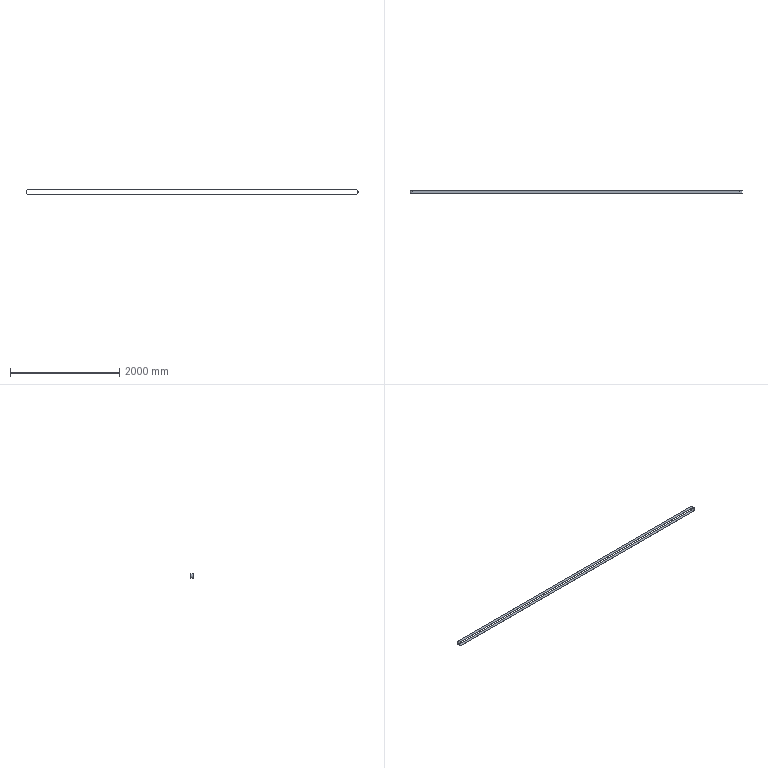Part | STEP file | HABASIT_ESTEIRA | 1 solid | 10 faces | box 6090 x 50 x 90 mm | volume 1227646 mm3 | plane 6 | cylinder 4 | commonest cylinder face diameters 86 x2 90 x2
STEP:
#1=CARTESIAN_POINT('',(0.,0.,0.));
#2=DIRECTION('',(0.,0.,1.));
#3=DIRECTION('',(1.,0.,0.));
#4=AXIS2_PLACEMENT_3D('',#1,#2,#3);
#5=CARTESIAN_POINT('',(0.,125.,-45.));
#6=VERTEX_POINT('',#5);
#7=CARTESIAN_POINT('',(0.,75.,-45.));
#8=VERTEX_POINT('',#7);
#9=CARTESIAN_POINT('',(0.,125.,-45.));
#10=DIRECTION('',(0.,-1.,0.));
#11=VECTOR('',#10,1.);
#12=LINE('',#9,#11);
#13=CARTESIAN_POINT('',(0.,125.,-45.));
#14=DIRECTION('',(0.,0.,-1.));
#15=DIRECTION('',(-1.,0.,0.));
#16=AXIS2_PLACEMENT_3D('',#13,#14,#15);
#17=PLANE('',#16);
#18=CARTESIAN_POINT('',(0.,0.));
#19=DIRECTION('',(0.,-1.));
#20=VECTOR('',#19,1.);
#21=LINE('',#18,#20);
#22=(GEOMETRIC_REPRESENTATION_CONTEXT(2)PARAMETRIC_REPRESENTATION_CONTEXT()REPRESENTATION_CONTEXT('',''));
#23=DEFINITIONAL_REPRESENTATION('',(#21),#22);
#24=PCURVE('',#17,#23);
#25=CARTESIAN_POINT('',(0.,100.,0.));
#26=DIRECTION('',(0.,1.,0.));
#27=DIRECTION('',(0.,0.,-1.));
#28=AXIS2_PLACEMENT_3D('',#25,#26,#27);
#29=CYLINDRICAL_SURFACE('',#28,45.);
#30=CARTESIAN_POINT('',(0.,25.));
#31=DIRECTION('',(0.,-1.));
#32=VECTOR('',#31,1.);
#33=LINE('',#30,#32);
#34=(GEOMETRIC_REPRESENTATION_CONTEXT(2)PARAMETRIC_REPRESENTATION_CONTEXT()REPRESENTATION_CONTEXT('',''));
#35=DEFINITIONAL_REPRESENTATION('',(#33),#34);
#36=PCURVE('',#29,#35);
#37=SURFACE_CURVE('',#12,(#24,#36),.PCURVE_S1.);
#38=EDGE_CURVE('',#6,#8,#37,.T.);
#39=ORIENTED_EDGE('',*,*,#38,.F.);
#40=CARTESIAN_POINT('',(6000.,125.,-45.));
#41=VERTEX_POINT('',#40);
#42=CARTESIAN_POINT('',(0.,125.,-45.));
#43=DIRECTION('',(1.,0.,0.));
#44=VECTOR('',#43,1.);
#45=LINE('',#42,#44);
#46=CARTESIAN_POINT('',(0.,0.));
#47=DIRECTION('',(-1.,0.));
#48=VECTOR('',#47,1.);
#49=LINE('',#46,#48);
#50=(GEOMETRIC_REPRESENTATION_CONTEXT(2)PARAMETRIC_REPRESENTATION_CONTEXT()REPRESENTATION_CONTEXT('',''));
#51=DEFINITIONAL_REPRESENTATION('',(#49),#50);
#52=PCURVE('',#17,#51);
#53=CARTESIAN_POINT('',(0.,125.,0.));
#54=DIRECTION('',(0.,1.,0.));
#55=DIRECTION('',(0.,0.,1.));
#56=AXIS2_PLACEMENT_3D('',#53,#54,#55);
#57=PLANE('',#56);
#58=CARTESIAN_POINT('',(-45.,0.));
#59=DIRECTION('',(0.,1.));
#60=VECTOR('',#59,1.);
#61=LINE('',#58,#60);
#62=(GEOMETRIC_REPRESENTATION_CONTEXT(2)PARAMETRIC_REPRESENTATION_CONTEXT()REPRESENTATION_CONTEXT('',''));
#63=DEFINITIONAL_REPRESENTATION('',(#61),#62);
#64=PCURVE('',#57,#63);
#65=SURFACE_CURVE('',#45,(#52,#64),.PCURVE_S1.);
#66=EDGE_CURVE('',#6,#41,#65,.T.);
#67=ORIENTED_EDGE('',*,*,#66,.T.);
#68=CARTESIAN_POINT('',(6000.,75.,-45.));
#69=VERTEX_POINT('',#68);
#70=CARTESIAN_POINT('',(6000.,125.,-45.));
#71=DIRECTION('',(0.,-1.,0.));
#72=VECTOR('',#71,1.);
#73=LINE('',#70,#72);
#74=CARTESIAN_POINT('',(-6000.,0.));
#75=DIRECTION('',(0.,-1.));
#76=VECTOR('',#75,1.);
#77=LINE('',#74,#76);
#78=(GEOMETRIC_REPRESENTATION_CONTEXT(2)PARAMETRIC_REPRESENTATION_CONTEXT()REPRESENTATION_CONTEXT('',''));
#79=DEFINITIONAL_REPRESENTATION('',(#77),#78);
#80=PCURVE('',#17,#79);
#81=CARTESIAN_POINT('',(6000.,100.,0.));
#82=DIRECTION('',(0.,1.,0.));
#83=DIRECTION('',(0.,0.,1.));
#84=AXIS2_PLACEMENT_3D('',#81,#82,#83);
#85=CYLINDRICAL_SURFACE('',#84,45.);
#86=CARTESIAN_POINT('',(3.142,25.));
#87=DIRECTION('',(0.,-1.));
#88=VECTOR('',#87,1.);
#89=LINE('',#86,#88);
#90=(GEOMETRIC_REPRESENTATION_CONTEXT(2)PARAMETRIC_REPRESENTATION_CONTEXT()REPRESENTATION_CONTEXT('',''));
#91=DEFINITIONAL_REPRESENTATION('',(#89),#90);
#92=PCURVE('',#85,#91);
#93=SURFACE_CURVE('',#73,(#80,#92),.PCURVE_S1.);
#94=EDGE_CURVE('',#41,#69,#93,.T.);
#95=ORIENTED_EDGE('',*,*,#94,.T.);
#96=CARTESIAN_POINT('',(0.,75.,-45.));
#97=DIRECTION('',(1.,0.,0.));
#98=VECTOR('',#97,1.);
#99=LINE('',#96,#98);
#100=CARTESIAN_POINT('',(0.,-50.));
#101=DIRECTION('',(-1.,0.));
#102=VECTOR('',#101,1.);
#103=LINE('',#100,#102);
#104=(GEOMETRIC_REPRESENTATION_CONTEXT(2)PARAMETRIC_REPRESENTATION_CONTEXT()REPRESENTATION_CONTEXT('',''));
#105=DEFINITIONAL_REPRESENTATION('',(#103),#104);
#106=PCURVE('',#17,#105);
#107=CARTESIAN_POINT('',(0.,75.,0.));
#108=DIRECTION('',(0.,1.,0.));
#109=DIRECTION('',(0.,0.,1.));
#110=AXIS2_PLACEMENT_3D('',#107,#108,#109);
#111=PLANE('',#110);
#112=CARTESIAN_POINT('',(-45.,0.));
#113=DIRECTION('',(0.,1.));
#114=VECTOR('',#113,1.);
#115=LINE('',#112,#114);
#116=(GEOMETRIC_REPRESENTATION_CONTEXT(2)PARAMETRIC_REPRESENTATION_CONTEXT()REPRESENTATION_CONTEXT('',''));
#117=DEFINITIONAL_REPRESENTATION('',(#115),#116);
#118=PCURVE('',#111,#117);
#119=SURFACE_CURVE('',#99,(#106,#118),.PCURVE_S1.);
#120=EDGE_CURVE('',#8,#69,#119,.T.);
#121=ORIENTED_EDGE('',*,*,#120,.F.);
#122=EDGE_LOOP('',(#39,#67,#95,#121));
#123=FACE_BOUND('',#122,.T.);
#124=ADVANCED_FACE('',(#123),#17,.T.);
#125=CARTESIAN_POINT('',(0.,75.,45.));
#126=VERTEX_POINT('',#125);
#127=CARTESIAN_POINT('',(0.,75.,0.));
#128=DIRECTION('',(0.,1.,0.));
#129=DIRECTION('',(1.,0.,0.));
#130=AXIS2_PLACEMENT_3D('',#127,#128,#129);
#131=CIRCLE('',#130,45.);
#132=CARTESIAN_POINT('',(-1.571,-25.));
#133=DIRECTION('',(1.,0.));
#134=VECTOR('',#133,1.);
#135=LINE('',#132,#134);
#136=(GEOMETRIC_REPRESENTATION_CONTEXT(2)PARAMETRIC_REPRESENTATION_CONTEXT()REPRESENTATION_CONTEXT('',''));
#137=DEFINITIONAL_REPRESENTATION('',(#135),#136);
#138=PCURVE('',#29,#137);
#139=CARTESIAN_POINT('',(0.,0.));
#140=DIRECTION('',(0.,1.));
#141=AXIS2_PLACEMENT_2D('',#139,#140);
#142=CIRCLE('',#141,45.);
#143=(GEOMETRIC_REPRESENTATION_CONTEXT(2)PARAMETRIC_REPRESENTATION_CONTEXT()REPRESENTATION_CONTEXT('',''));
#144=DEFINITIONAL_REPRESENTATION('',(#142),#143);
#145=PCURVE('',#111,#144);
#146=SURFACE_CURVE('',#131,(#138,#145),.PCURVE_S1.);
#147=EDGE_CURVE('',#8,#126,#146,.T.);
#148=ORIENTED_EDGE('',*,*,#147,.T.);
#149=CARTESIAN_POINT('',(0.,125.,45.));
#150=VERTEX_POINT('',#149);
#151=CARTESIAN_POINT('',(0.,75.,45.));
#152=DIRECTION('',(0.,1.,0.));
#153=VECTOR('',#152,1.);
#154=LINE('',#151,#153);
#155=CARTESIAN_POINT('',(3.142,-25.));
#156=DIRECTION('',(0.,1.));
#157=VECTOR('',#156,1.);
#158=LINE('',#155,#157);
#159=(GEOMETRIC_REPRESENTATION_CONTEXT(2)PARAMETRIC_REPRESENTATION_CONTEXT()REPRESENTATION_CONTEXT('',''));
#160=DEFINITIONAL_REPRESENTATION('',(#158),#159);
#161=PCURVE('',#29,#160);
#162=CARTESIAN_POINT('',(6000.,125.,45.));
#163=DIRECTION('',(0.,0.,1.));
#164=DIRECTION('',(1.,0.,0.));
#165=AXIS2_PLACEMENT_3D('',#162,#163,#164);
#166=PLANE('',#165);
#167=CARTESIAN_POINT('',(-6000.,-50.));
#168=DIRECTION('',(0.,1.));
#169=VECTOR('',#168,1.);
#170=LINE('',#167,#169);
#171=(GEOMETRIC_REPRESENTATION_CONTEXT(2)PARAMETRIC_REPRESENTATION_CONTEXT()REPRESENTATION_CONTEXT('',''));
#172=DEFINITIONAL_REPRESENTATION('',(#170),#171);
#173=PCURVE('',#166,#172);
#174=SURFACE_CURVE('',#154,(#161,#173),.PCURVE_S1.);
#175=EDGE_CURVE('',#126,#150,#174,.T.);
#176=ORIENTED_EDGE('',*,*,#175,.T.);
#177=CARTESIAN_POINT('',(0.,125.,0.));
#178=DIRECTION('',(0.,1.,0.));
#179=DIRECTION('',(1.,0.,0.));
#180=AXIS2_PLACEMENT_3D('',#177,#178,#179);
#181=CIRCLE('',#180,45.);
#182=CARTESIAN_POINT('',(-1.571,25.));
#183=DIRECTION('',(1.,0.));
#184=VECTOR('',#183,1.);
#185=LINE('',#182,#184);
#186=(GEOMETRIC_REPRESENTATION_CONTEXT(2)PARAMETRIC_REPRESENTATION_CONTEXT()REPRESENTATION_CONTEXT('',''));
#187=DEFINITIONAL_REPRESENTATION('',(#185),#186);
#188=PCURVE('',#29,#187);
#189=CARTESIAN_POINT('',(0.,0.));
#190=DIRECTION('',(0.,1.));
#191=AXIS2_PLACEMENT_2D('',#189,#190);
#192=CIRCLE('',#191,45.);
#193=(GEOMETRIC_REPRESENTATION_CONTEXT(2)PARAMETRIC_REPRESENTATION_CONTEXT()REPRESENTATION_CONTEXT('',''));
#194=DEFINITIONAL_REPRESENTATION('',(#192),#193);
#195=PCURVE('',#57,#194);
#196=SURFACE_CURVE('',#181,(#188,#195),.PCURVE_S1.);
#197=EDGE_CURVE('',#6,#150,#196,.T.);
#198=ORIENTED_EDGE('',*,*,#197,.F.);
#199=ORIENTED_EDGE('',*,*,#38,.T.);
#200=EDGE_LOOP('',(#148,#176,#198,#199));
#201=FACE_BOUND('',#200,.T.);
#202=ADVANCED_FACE('',(#201),#29,.T.);
#203=CARTESIAN_POINT('',(6000.,125.,45.));
#204=VERTEX_POINT('',#203);
#205=CARTESIAN_POINT('',(6000.,75.,45.));
#206=VERTEX_POINT('',#205);
#207=CARTESIAN_POINT('',(6000.,125.,45.));
#208=DIRECTION('',(0.,-1.,0.));
#209=VECTOR('',#208,1.);
#210=LINE('',#207,#209);
#211=CARTESIAN_POINT('',(0.,0.));
#212=DIRECTION('',(0.,-1.));
#213=VECTOR('',#212,1.);
#214=LINE('',#211,#213);
#215=(GEOMETRIC_REPRESENTATION_CONTEXT(2)PARAMETRIC_REPRESENTATION_CONTEXT()REPRESENTATION_CONTEXT('',''));
#216=DEFINITIONAL_REPRESENTATION('',(#214),#215);
#217=PCURVE('',#166,#216);
#218=CARTESIAN_POINT('',(0.,25.));
#219=DIRECTION('',(0.,-1.));
#220=VECTOR('',#219,1.);
#221=LINE('',#218,#220);
#222=(GEOMETRIC_REPRESENTATION_CONTEXT(2)PARAMETRIC_REPRESENTATION_CONTEXT()REPRESENTATION_CONTEXT('',''));
#223=DEFINITIONAL_REPRESENTATION('',(#221),#222);
#224=PCURVE('',#85,#223);
#225=SURFACE_CURVE('',#210,(#217,#224),.PCURVE_S1.);
#226=EDGE_CURVE('',#204,#206,#225,.T.);
#227=ORIENTED_EDGE('',*,*,#226,.F.);
#228=CARTESIAN_POINT('',(6000.,125.,45.));
#229=DIRECTION('',(-1.,0.,0.));
#230=VECTOR('',#229,1.);
#231=LINE('',#228,#230);
#232=CARTESIAN_POINT('',(0.,0.));
#233=DIRECTION('',(-1.,0.));
#234=VECTOR('',#233,1.);
#235=LINE('',#232,#234);
#236=(GEOMETRIC_REPRESENTATION_CONTEXT(2)PARAMETRIC_REPRESENTATION_CONTEXT()REPRESENTATION_CONTEXT('',''));
#237=DEFINITIONAL_REPRESENTATION('',(#235),#236);
#238=PCURVE('',#166,#237);
#239=CARTESIAN_POINT('',(45.,6000.));
#240=DIRECTION('',(0.,-1.));
#241=VECTOR('',#240,1.);
#242=LINE('',#239,#241);
#243=(GEOMETRIC_REPRESENTATION_CONTEXT(2)PARAMETRIC_REPRESENTATION_CONTEXT()REPRESENTATION_CONTEXT('',''));
#244=DEFINITIONAL_REPRESENTATION('',(#242),#243);
#245=PCURVE('',#57,#244);
#246=SURFACE_CURVE('',#231,(#238,#245),.PCURVE_S1.);
#247=EDGE_CURVE('',#204,#150,#246,.T.);
#248=ORIENTED_EDGE('',*,*,#247,.T.);
#249=ORIENTED_EDGE('',*,*,#175,.F.);
#250=CARTESIAN_POINT('',(6000.,75.,45.));
#251=DIRECTION('',(-1.,0.,0.));
#252=VECTOR('',#251,1.);
#253=LINE('',#250,#252);
#254=CARTESIAN_POINT('',(0.,-50.));
#255=DIRECTION('',(-1.,0.));
#256=VECTOR('',#255,1.);
#257=LINE('',#254,#256);
#258=(GEOMETRIC_REPRESENTATION_CONTEXT(2)PARAMETRIC_REPRESENTATION_CONTEXT()REPRESENTATION_CONTEXT('',''));
#259=DEFINITIONAL_REPRESENTATION('',(#257),#258);
#260=PCURVE('',#166,#259);
#261=CARTESIAN_POINT('',(45.,6000.));
#262=DIRECTION('',(0.,-1.));
#263=VECTOR('',#262,1.);
#264=LINE('',#261,#263);
#265=(GEOMETRIC_REPRESENTATION_CONTEXT(2)PARAMETRIC_REPRESENTATION_CONTEXT()REPRESENTATION_CONTEXT('',''));
#266=DEFINITIONAL_REPRESENTATION('',(#264),#265);
#267=PCURVE('',#111,#266);
#268=SURFACE_CURVE('',#253,(#260,#267),.PCURVE_S1.);
#269=EDGE_CURVE('',#206,#126,#268,.T.);
#270=ORIENTED_EDGE('',*,*,#269,.F.);
#271=EDGE_LOOP('',(#227,#248,#249,#270));
#272=FACE_BOUND('',#271,.T.);
#273=ADVANCED_FACE('',(#272),#166,.T.);
#274=CARTESIAN_POINT('',(6000.,75.,0.));
#275=DIRECTION('',(0.,1.,0.));
#276=DIRECTION('',(1.,0.,0.));
#277=AXIS2_PLACEMENT_3D('',#274,#275,#276);
#278=CIRCLE('',#277,45.);
#279=CARTESIAN_POINT('',(-4.712,-25.));
#280=DIRECTION('',(1.,0.));
#281=VECTOR('',#280,1.);
#282=LINE('',#279,#281);
#283=(GEOMETRIC_REPRESENTATION_CONTEXT(2)PARAMETRIC_REPRESENTATION_CONTEXT()REPRESENTATION_CONTEXT('',''));
#284=DEFINITIONAL_REPRESENTATION('',(#282),#283);
#285=PCURVE('',#85,#284);
#286=CARTESIAN_POINT('',(0.,6000.));
#287=DIRECTION('',(0.,1.));
#288=AXIS2_PLACEMENT_2D('',#286,#287);
#289=CIRCLE('',#288,45.);
#290=(GEOMETRIC_REPRESENTATION_CONTEXT(2)PARAMETRIC_REPRESENTATION_CONTEXT()REPRESENTATION_CONTEXT('',''));
#291=DEFINITIONAL_REPRESENTATION('',(#289),#290);
#292=PCURVE('',#111,#291);
#293=SURFACE_CURVE('',#278,(#285,#292),.PCURVE_S1.);
#294=EDGE_CURVE('',#206,#69,#293,.T.);
#295=ORIENTED_EDGE('',*,*,#294,.T.);
#296=ORIENTED_EDGE('',*,*,#94,.F.);
#297=CARTESIAN_POINT('',(6000.,125.,0.));
#298=DIRECTION('',(0.,1.,0.));
#299=DIRECTION('',(1.,0.,0.));
#300=AXIS2_PLACEMENT_3D('',#297,#298,#299);
#301=CIRCLE('',#300,45.);
#302=CARTESIAN_POINT('',(-4.712,25.));
#303=DIRECTION('',(1.,0.));
#304=VECTOR('',#303,1.);
#305=LINE('',#302,#304);
#306=(GEOMETRIC_REPRESENTATION_CONTEXT(2)PARAMETRIC_REPRESENTATION_CONTEXT()REPRESENTATION_CONTEXT('',''));
#307=DEFINITIONAL_REPRESENTATION('',(#305),#306);
#308=PCURVE('',#85,#307);
#309=CARTESIAN_POINT('',(0.,6000.));
#310=DIRECTION('',(0.,1.));
#311=AXIS2_PLACEMENT_2D('',#309,#310);
#312=CIRCLE('',#311,45.);
#313=(GEOMETRIC_REPRESENTATION_CONTEXT(2)PARAMETRIC_REPRESENTATION_CONTEXT()REPRESENTATION_CONTEXT('',''));
#314=DEFINITIONAL_REPRESENTATION('',(#312),#313);
#315=PCURVE('',#57,#314);
#316=SURFACE_CURVE('',#301,(#308,#315),.PCURVE_S1.);
#317=EDGE_CURVE('',#204,#41,#316,.T.);
#318=ORIENTED_EDGE('',*,*,#317,.F.);
#319=ORIENTED_EDGE('',*,*,#226,.T.);
#320=EDGE_LOOP('',(#295,#296,#318,#319));
#321=FACE_BOUND('',#320,.T.);
#322=ADVANCED_FACE('',(#321),#85,.T.);
#323=CARTESIAN_POINT('',(0.,75.,-43.));
#324=VERTEX_POINT('',#323);
#325=CARTESIAN_POINT('',(6000.,75.,-43.));
#326=VERTEX_POINT('',#325);
#327=CARTESIAN_POINT('',(0.,75.,-43.));
#328=DIRECTION('',(1.,0.,0.));
#329=VECTOR('',#328,1.);
#330=LINE('',#327,#329);
#331=CARTESIAN_POINT('',(0.,125.,-43.));
#332=DIRECTION('',(0.,0.,-1.));
#333=DIRECTION('',(-1.,0.,0.));
#334=AXIS2_PLACEMENT_3D('',#331,#332,#333);
#335=PLANE('',#334);
#336=CARTESIAN_POINT('',(0.,-50.));
#337=DIRECTION('',(-1.,0.));
#338=VECTOR('',#337,1.);
#339=LINE('',#336,#338);
#340=(GEOMETRIC_REPRESENTATION_CONTEXT(2)PARAMETRIC_REPRESENTATION_CONTEXT()REPRESENTATION_CONTEXT('',''));
#341=DEFINITIONAL_REPRESENTATION('',(#339),#340);
#342=PCURVE('',#335,#341);
#343=CARTESIAN_POINT('',(-43.,0.));
#344=DIRECTION('',(0.,1.));
#345=VECTOR('',#344,1.);
#346=LINE('',#343,#345);
#347=(GEOMETRIC_REPRESENTATION_CONTEXT(2)PARAMETRIC_REPRESENTATION_CONTEXT()REPRESENTATION_CONTEXT('',''));
#348=DEFINITIONAL_REPRESENTATION('',(#346),#347);
#349=PCURVE('',#111,#348);
#350=SURFACE_CURVE('',#330,(#342,#349),.PCURVE_S1.);
#351=EDGE_CURVE('',#324,#326,#350,.T.);
#352=ORIENTED_EDGE('',*,*,#351,.T.);
#353=CARTESIAN_POINT('',(6000.,125.,-43.));
#354=VERTEX_POINT('',#353);
#355=CARTESIAN_POINT('',(6000.,125.,-43.));
#356=DIRECTION('',(0.,-1.,0.));
#357=VECTOR('',#356,1.);
#358=LINE('',#355,#357);
#359=CARTESIAN_POINT('',(-6000.,0.));
#360=DIRECTION('',(0.,-1.));
#361=VECTOR('',#360,1.);
#362=LINE('',#359,#361);
#363=(GEOMETRIC_REPRESENTATION_CONTEXT(2)PARAMETRIC_REPRESENTATION_CONTEXT()REPRESENTATION_CONTEXT('',''));
#364=DEFINITIONAL_REPRESENTATION('',(#362),#363);
#365=PCURVE('',#335,#364);
#366=CARTESIAN_POINT('',(6000.,100.,0.));
#367=DIRECTION('',(0.,1.,0.));
#368=DIRECTION('',(0.,0.,1.));
#369=AXIS2_PLACEMENT_3D('',#366,#367,#368);
#370=CYLINDRICAL_SURFACE('',#369,43.);
#371=CARTESIAN_POINT('',(3.142,25.));
#372=DIRECTION('',(0.,-1.));
#373=VECTOR('',#372,1.);
#374=LINE('',#371,#373);
#375=(GEOMETRIC_REPRESENTATION_CONTEXT(2)PARAMETRIC_REPRESENTATION_CONTEXT()REPRESENTATION_CONTEXT('',''));
#376=DEFINITIONAL_REPRESENTATION('',(#374),#375);
#377=PCURVE('',#370,#376);
#378=SURFACE_CURVE('',#358,(#365,#377),.PCURVE_S1.);
#379=EDGE_CURVE('',#354,#326,#378,.T.);
#380=ORIENTED_EDGE('',*,*,#379,.F.);
#381=CARTESIAN_POINT('',(0.,125.,-43.));
#382=VERTEX_POINT('',#381);
#383=CARTESIAN_POINT('',(0.,125.,-43.));
#384=DIRECTION('',(1.,0.,0.));
#385=VECTOR('',#384,1.);
#386=LINE('',#383,#385);
#387=CARTESIAN_POINT('',(0.,0.));
#388=DIRECTION('',(-1.,0.));
#389=VECTOR('',#388,1.);
#390=LINE('',#387,#389);
#391=(GEOMETRIC_REPRESENTATION_CONTEXT(2)PARAMETRIC_REPRESENTATION_CONTEXT()REPRESENTATION_CONTEXT('',''));
#392=DEFINITIONAL_REPRESENTATION('',(#390),#391);
#393=PCURVE('',#335,#392);
#394=CARTESIAN_POINT('',(-43.,0.));
#395=DIRECTION('',(0.,1.));
#396=VECTOR('',#395,1.);
#397=LINE('',#394,#396);
#398=(GEOMETRIC_REPRESENTATION_CONTEXT(2)PARAMETRIC_REPRESENTATION_CONTEXT()REPRESENTATION_CONTEXT('',''));
#399=DEFINITIONAL_REPRESENTATION('',(#397),#398);
#400=PCURVE('',#57,#399);
#401=SURFACE_CURVE('',#386,(#393,#400),.PCURVE_S1.);
#402=EDGE_CURVE('',#382,#354,#401,.T.);
#403=ORIENTED_EDGE('',*,*,#402,.F.);
#404=CARTESIAN_POINT('',(0.,125.,-43.));
#405=DIRECTION('',(0.,-1.,0.));
#406=VECTOR('',#405,1.);
#407=LINE('',#404,#406);
#408=CARTESIAN_POINT('',(0.,0.));
#409=DIRECTION('',(0.,-1.));
#410=VECTOR('',#409,1.);
#411=LINE('',#408,#410);
#412=(GEOMETRIC_REPRESENTATION_CONTEXT(2)PARAMETRIC_REPRESENTATION_CONTEXT()REPRESENTATION_CONTEXT('',''));
#413=DEFINITIONAL_REPRESENTATION('',(#411),#412);
#414=PCURVE('',#335,#413);
#415=CARTESIAN_POINT('',(0.,100.,0.));
#416=DIRECTION('',(0.,1.,0.));
#417=DIRECTION('',(0.,0.,-1.));
#418=AXIS2_PLACEMENT_3D('',#415,#416,#417);
#419=CYLINDRICAL_SURFACE('',#418,43.);
#420=CARTESIAN_POINT('',(0.,25.));
#421=DIRECTION('',(0.,-1.));
#422=VECTOR('',#421,1.);
#423=LINE('',#420,#422);
#424=(GEOMETRIC_REPRESENTATION_CONTEXT(2)PARAMETRIC_REPRESENTATION_CONTEXT()REPRESENTATION_CONTEXT('',''));
#425=DEFINITIONAL_REPRESENTATION('',(#423),#424);
#426=PCURVE('',#419,#425);
#427=SURFACE_CURVE('',#407,(#414,#426),.PCURVE_S1.);
#428=EDGE_CURVE('',#382,#324,#427,.T.);
#429=ORIENTED_EDGE('',*,*,#428,.T.);
#430=EDGE_LOOP('',(#352,#380,#403,#429));
#431=FACE_BOUND('',#430,.T.);
#432=ADVANCED_FACE('',(#431),#335,.F.);
#433=CARTESIAN_POINT('',(6000.,75.,43.));
#434=VERTEX_POINT('',#433);
#435=CARTESIAN_POINT('',(6000.,75.,0.));
#436=DIRECTION('',(0.,1.,0.));
#437=DIRECTION('',(1.,0.,0.));
#438=AXIS2_PLACEMENT_3D('',#435,#436,#437);
#439=CIRCLE('',#438,43.);
#440=CARTESIAN_POINT('',(-4.712,-25.));
#441=DIRECTION('',(1.,0.));
#442=VECTOR('',#441,1.);
#443=LINE('',#440,#442);
#444=(GEOMETRIC_REPRESENTATION_CONTEXT(2)PARAMETRIC_REPRESENTATION_CONTEXT()REPRESENTATION_CONTEXT('',''));
#445=DEFINITIONAL_REPRESENTATION('',(#443),#444);
#446=PCURVE('',#370,#445);
#447=CARTESIAN_POINT('',(0.,6000.));
#448=DIRECTION('',(0.,1.));
#449=AXIS2_PLACEMENT_2D('',#447,#448);
#450=CIRCLE('',#449,43.);
#451=(GEOMETRIC_REPRESENTATION_CONTEXT(2)PARAMETRIC_REPRESENTATION_CONTEXT()REPRESENTATION_CONTEXT('',''));
#452=DEFINITIONAL_REPRESENTATION('',(#450),#451);
#453=PCURVE('',#111,#452);
#454=SURFACE_CURVE('',#439,(#446,#453),.PCURVE_S1.);
#455=EDGE_CURVE('',#434,#326,#454,.T.);
#456=ORIENTED_EDGE('',*,*,#455,.T.);
#457=ORIENTED_EDGE('',*,*,#379,.F.);
#458=CARTESIAN_POINT('',(6000.,125.,43.));
#459=VERTEX_POINT('',#458);
#460=CARTESIAN_POINT('',(6000.,125.,0.));
#461=DIRECTION('',(0.,1.,0.));
#462=DIRECTION('',(1.,0.,0.));
#463=AXIS2_PLACEMENT_3D('',#460,#461,#462);
#464=CIRCLE('',#463,43.);
#465=CARTESIAN_POINT('',(-4.712,25.));
#466=DIRECTION('',(1.,0.));
#467=VECTOR('',#466,1.);
#468=LINE('',#465,#467);
#469=(GEOMETRIC_REPRESENTATION_CONTEXT(2)PARAMETRIC_REPRESENTATION_CONTEXT()REPRESENTATION_CONTEXT('',''));
#470=DEFINITIONAL_REPRESENTATION('',(#468),#469);
#471=PCURVE('',#370,#470);
#472=CARTESIAN_POINT('',(0.,6000.));
#473=DIRECTION('',(0.,1.));
#474=AXIS2_PLACEMENT_2D('',#472,#473);
#475=CIRCLE('',#474,43.);
#476=(GEOMETRIC_REPRESENTATION_CONTEXT(2)PARAMETRIC_REPRESENTATION_CONTEXT()REPRESENTATION_CONTEXT('',''));
#477=DEFINITIONAL_REPRESENTATION('',(#475),#476);
#478=PCURVE('',#57,#477);
#479=SURFACE_CURVE('',#464,(#471,#478),.PCURVE_S1.);
#480=EDGE_CURVE('',#459,#354,#479,.T.);
#481=ORIENTED_EDGE('',*,*,#480,.F.);
#482=CARTESIAN_POINT('',(6000.,75.,43.));
#483=DIRECTION('',(0.,1.,0.));
#484=VECTOR('',#483,1.);
#485=LINE('',#482,#484);
#486=CARTESIAN_POINT('',(0.,-25.));
#487=DIRECTION('',(0.,1.));
#488=VECTOR('',#487,1.);
#489=LINE('',#486,#488);
#490=(GEOMETRIC_REPRESENTATION_CONTEXT(2)PARAMETRIC_REPRESENTATION_CONTEXT()REPRESENTATION_CONTEXT('',''));
#491=DEFINITIONAL_REPRESENTATION('',(#489),#490);
#492=PCURVE('',#370,#491);
#493=CARTESIAN_POINT('',(6000.,125.,43.));
#494=DIRECTION('',(0.,0.,1.));
#495=DIRECTION('',(1.,0.,0.));
#496=AXIS2_PLACEMENT_3D('',#493,#494,#495);
#497=PLANE('',#496);
#498=CARTESIAN_POINT('',(0.,-50.));
#499=DIRECTION('',(0.,1.));
#500=VECTOR('',#499,1.);
#501=LINE('',#498,#500);
#502=(GEOMETRIC_REPRESENTATION_CONTEXT(2)PARAMETRIC_REPRESENTATION_CONTEXT()REPRESENTATION_CONTEXT('',''));
#503=DEFINITIONAL_REPRESENTATION('',(#501),#502);
#504=PCURVE('',#497,#503);
#505=SURFACE_CURVE('',#485,(#492,#504),.PCURVE_S1.);
#506=EDGE_CURVE('',#434,#459,#505,.T.);
#507=ORIENTED_EDGE('',*,*,#506,.F.);
#508=EDGE_LOOP('',(#456,#457,#481,#507));
#509=FACE_BOUND('',#508,.F.);
#510=ADVANCED_FACE('',(#509),#370,.F.);
#511=CARTESIAN_POINT('',(0.,75.,43.));
#512=VERTEX_POINT('',#511);
#513=CARTESIAN_POINT('',(6000.,75.,43.));
#514=DIRECTION('',(-1.,0.,0.));
#515=VECTOR('',#514,1.);
#516=LINE('',#513,#515);
#517=CARTESIAN_POINT('',(0.,-50.));
#518=DIRECTION('',(-1.,0.));
#519=VECTOR('',#518,1.);
#520=LINE('',#517,#519);
#521=(GEOMETRIC_REPRESENTATION_CONTEXT(2)PARAMETRIC_REPRESENTATION_CONTEXT()REPRESENTATION_CONTEXT('',''));
#522=DEFINITIONAL_REPRESENTATION('',(#520),#521);
#523=PCURVE('',#497,#522);
#524=CARTESIAN_POINT('',(43.,6000.));
#525=DIRECTION('',(0.,-1.));
#526=VECTOR('',#525,1.);
#527=LINE('',#524,#526);
#528=(GEOMETRIC_REPRESENTATION_CONTEXT(2)PARAMETRIC_REPRESENTATION_CONTEXT()REPRESENTATION_CONTEXT('',''));
#529=DEFINITIONAL_REPRESENTATION('',(#527),#528);
#530=PCURVE('',#111,#529);
#531=SURFACE_CURVE('',#516,(#523,#530),.PCURVE_S1.);
#532=EDGE_CURVE('',#434,#512,#531,.T.);
#533=ORIENTED_EDGE('',*,*,#532,.T.);
#534=CARTESIAN_POINT('',(0.,125.,43.));
#535=VERTEX_POINT('',#534);
#536=CARTESIAN_POINT('',(0.,125.,43.));
#537=DIRECTION('',(0.,-1.,0.));
#538=VECTOR('',#537,1.);
#539=LINE('',#536,#538);
#540=CARTESIAN_POINT('',(-6000.,0.));
#541=DIRECTION('',(0.,-1.));
#542=VECTOR('',#541,1.);
#543=LINE('',#540,#542);
#544=(GEOMETRIC_REPRESENTATION_CONTEXT(2)PARAMETRIC_REPRESENTATION_CONTEXT()REPRESENTATION_CONTEXT('',''));
#545=DEFINITIONAL_REPRESENTATION('',(#543),#544);
#546=PCURVE('',#497,#545);
#547=CARTESIAN_POINT('',(3.142,25.));
#548=DIRECTION('',(0.,-1.));
#549=VECTOR('',#548,1.);
#550=LINE('',#547,#549);
#551=(GEOMETRIC_REPRESENTATION_CONTEXT(2)PARAMETRIC_REPRESENTATION_CONTEXT()REPRESENTATION_CONTEXT('',''));
#552=DEFINITIONAL_REPRESENTATION('',(#550),#551);
#553=PCURVE('',#419,#552);
#554=SURFACE_CURVE('',#539,(#546,#553),.PCURVE_S1.);
#555=EDGE_CURVE('',#535,#512,#554,.T.);
#556=ORIENTED_EDGE('',*,*,#555,.F.);
#557=CARTESIAN_POINT('',(6000.,125.,43.));
#558=DIRECTION('',(-1.,0.,0.));
#559=VECTOR('',#558,1.);
#560=LINE('',#557,#559);
#561=CARTESIAN_POINT('',(0.,0.));
#562=DIRECTION('',(-1.,0.));
#563=VECTOR('',#562,1.);
#564=LINE('',#561,#563);
#565=(GEOMETRIC_REPRESENTATION_CONTEXT(2)PARAMETRIC_REPRESENTATION_CONTEXT()REPRESENTATION_CONTEXT('',''));
#566=DEFINITIONAL_REPRESENTATION('',(#564),#565);
#567=PCURVE('',#497,#566);
#568=CARTESIAN_POINT('',(43.,6000.));
#569=DIRECTION('',(0.,-1.));
#570=VECTOR('',#569,1.);
#571=LINE('',#568,#570);
#572=(GEOMETRIC_REPRESENTATION_CONTEXT(2)PARAMETRIC_REPRESENTATION_CONTEXT()REPRESENTATION_CONTEXT('',''));
#573=DEFINITIONAL_REPRESENTATION('',(#571),#572);
#574=PCURVE('',#57,#573);
#575=SURFACE_CURVE('',#560,(#567,#574),.PCURVE_S1.);
#576=EDGE_CURVE('',#459,#535,#575,.T.);
#577=ORIENTED_EDGE('',*,*,#576,.F.);
#578=ORIENTED_EDGE('',*,*,#506,.F.);
#579=EDGE_LOOP('',(#533,#556,#577,#578));
#580=FACE_BOUND('',#579,.T.);
#581=ADVANCED_FACE('',(#580),#497,.F.);
#582=CARTESIAN_POINT('',(0.,75.,0.));
#583=DIRECTION('',(0.,1.,0.));
#584=DIRECTION('',(1.,0.,0.));
#585=AXIS2_PLACEMENT_3D('',#582,#583,#584);
#586=CIRCLE('',#585,43.);
#587=CARTESIAN_POINT('',(-1.571,-25.));
#588=DIRECTION('',(1.,0.));
#589=VECTOR('',#588,1.);
#590=LINE('',#587,#589);
#591=(GEOMETRIC_REPRESENTATION_CONTEXT(2)PARAMETRIC_REPRESENTATION_CONTEXT()REPRESENTATION_CONTEXT('',''));
#592=DEFINITIONAL_REPRESENTATION('',(#590),#591);
#593=PCURVE('',#419,#592);
#594=CARTESIAN_POINT('',(0.,0.));
#595=DIRECTION('',(0.,1.));
#596=AXIS2_PLACEMENT_2D('',#594,#595);
#597=CIRCLE('',#596,43.);
#598=(GEOMETRIC_REPRESENTATION_CONTEXT(2)PARAMETRIC_REPRESENTATION_CONTEXT()REPRESENTATION_CONTEXT('',''));
#599=DEFINITIONAL_REPRESENTATION('',(#597),#598);
#600=PCURVE('',#111,#599);
#601=SURFACE_CURVE('',#586,(#593,#600),.PCURVE_S1.);
#602=EDGE_CURVE('',#324,#512,#601,.T.);
#603=ORIENTED_EDGE('',*,*,#602,.T.);
#604=ORIENTED_EDGE('',*,*,#555,.F.);
#605=CARTESIAN_POINT('',(0.,125.,0.));
#606=DIRECTION('',(0.,1.,0.));
#607=DIRECTION('',(1.,0.,0.));
#608=AXIS2_PLACEMENT_3D('',#605,#606,#607);
#609=CIRCLE('',#608,43.);
#610=CARTESIAN_POINT('',(-1.571,25.));
#611=DIRECTION('',(1.,0.));
#612=VECTOR('',#611,1.);
#613=LINE('',#610,#612);
#614=(GEOMETRIC_REPRESENTATION_CONTEXT(2)PARAMETRIC_REPRESENTATION_CONTEXT()REPRESENTATION_CONTEXT('',''));
#615=DEFINITIONAL_REPRESENTATION('',(#613),#614);
#616=PCURVE('',#419,#615);
#617=CARTESIAN_POINT('',(0.,0.));
#618=DIRECTION('',(0.,1.));
#619=AXIS2_PLACEMENT_2D('',#617,#618);
#620=CIRCLE('',#619,43.);
#621=(GEOMETRIC_REPRESENTATION_CONTEXT(2)PARAMETRIC_REPRESENTATION_CONTEXT()REPRESENTATION_CONTEXT('',''));
#622=DEFINITIONAL_REPRESENTATION('',(#620),#621);
#623=PCURVE('',#57,#622);
#624=SURFACE_CURVE('',#609,(#616,#623),.PCURVE_S1.);
#625=EDGE_CURVE('',#382,#535,#624,.T.);
#626=ORIENTED_EDGE('',*,*,#625,.F.);
#627=ORIENTED_EDGE('',*,*,#428,.T.);
#628=EDGE_LOOP('',(#603,#604,#626,#627));
#629=FACE_BOUND('',#628,.F.);
#630=ADVANCED_FACE('',(#629),#419,.F.);
#631=ORIENTED_EDGE('',*,*,#66,.F.);
#632=ORIENTED_EDGE('',*,*,#197,.T.);
#633=ORIENTED_EDGE('',*,*,#247,.F.);
#634=ORIENTED_EDGE('',*,*,#317,.T.);
#635=EDGE_LOOP('',(#631,#632,#633,#634));
#636=FACE_BOUND('',#635,.T.);
#637=ORIENTED_EDGE('',*,*,#402,.T.);
#638=ORIENTED_EDGE('',*,*,#480,.F.);
#639=ORIENTED_EDGE('',*,*,#576,.T.);
#640=ORIENTED_EDGE('',*,*,#625,.F.);
#641=EDGE_LOOP('',(#637,#638,#639,#640));
#642=FACE_BOUND('',#641,.T.);
#643=ADVANCED_FACE('',(#636,#642),#57,.T.);
#644=ORIENTED_EDGE('',*,*,#294,.F.);
#645=ORIENTED_EDGE('',*,*,#269,.T.);
#646=ORIENTED_EDGE('',*,*,#147,.F.);
#647=ORIENTED_EDGE('',*,*,#120,.T.);
#648=EDGE_LOOP('',(#644,#645,#646,#647));
#649=FACE_BOUND('',#648,.T.);
#650=ORIENTED_EDGE('',*,*,#602,.T.);
#651=ORIENTED_EDGE('',*,*,#532,.F.);
#652=ORIENTED_EDGE('',*,*,#455,.T.);
#653=ORIENTED_EDGE('',*,*,#351,.F.);
#654=EDGE_LOOP('',(#650,#651,#652,#653));
#655=FACE_BOUND('',#654,.T.);
#656=ADVANCED_FACE('',(#649,#655),#111,.F.);
#657=CLOSED_SHELL('',(#124,#202,#273,#322,#432,#510,#581,#630,#643,#656));
#658=MANIFOLD_SOLID_BREP('',#657);
#659=(LENGTH_UNIT()NAMED_UNIT(*)SI_UNIT(.MILLI.,.METRE.));
#660=UNCERTAINTY_MEASURE_WITH_UNIT(LENGTH_MEASURE(0.0000001),#659,'','');
#661=(NAMED_UNIT(*)PLANE_ANGLE_UNIT()SI_UNIT($,.RADIAN.));
#662=(NAMED_UNIT(*)SI_UNIT($,.STERADIAN.)SOLID_ANGLE_UNIT());
#663=(GEOMETRIC_REPRESENTATION_CONTEXT(3)GLOBAL_UNCERTAINTY_ASSIGNED_CONTEXT((#660))GLOBAL_UNIT_ASSIGNED_CONTEXT((#659,#661,#662))REPRESENTATION_CONTEXT('',''));
#664=ADVANCED_BREP_SHAPE_REPRESENTATION('',(#4,#658),#663);